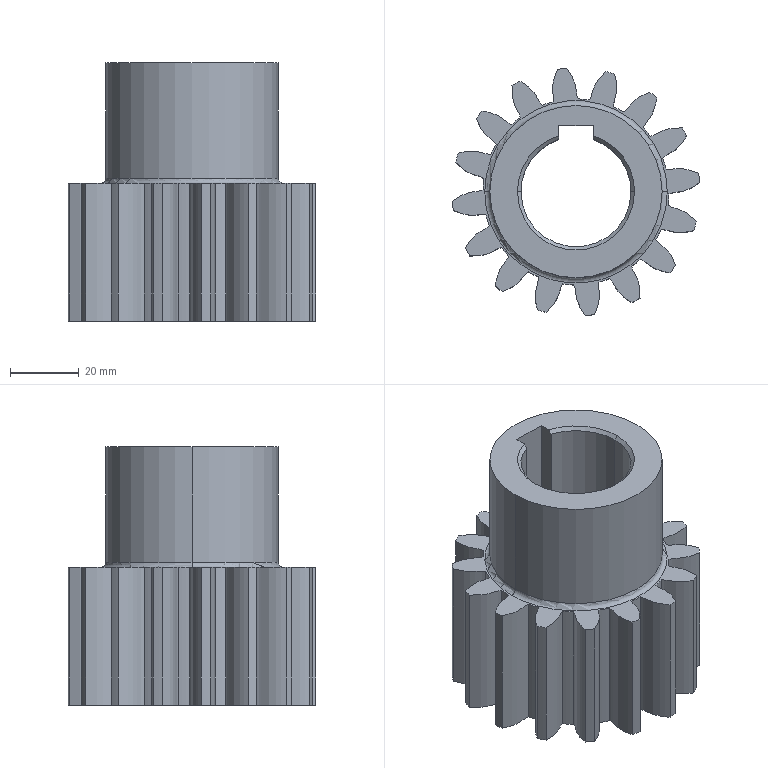Part | SolidWorks | features ICE 4, Chamfer 1, CirPattern 1, Extrusion 1, Fillet 1 | 1 solid | 88 faces | box 71.792 x 71.792 x 75 mm | volume 126582 mm3 | cylinder 39 | spline 32 | cone 8 | plane 7 | torus 2 | commonest cylinder face diameters 54 x16 72 x16 32 x3 42 x2 50 x2